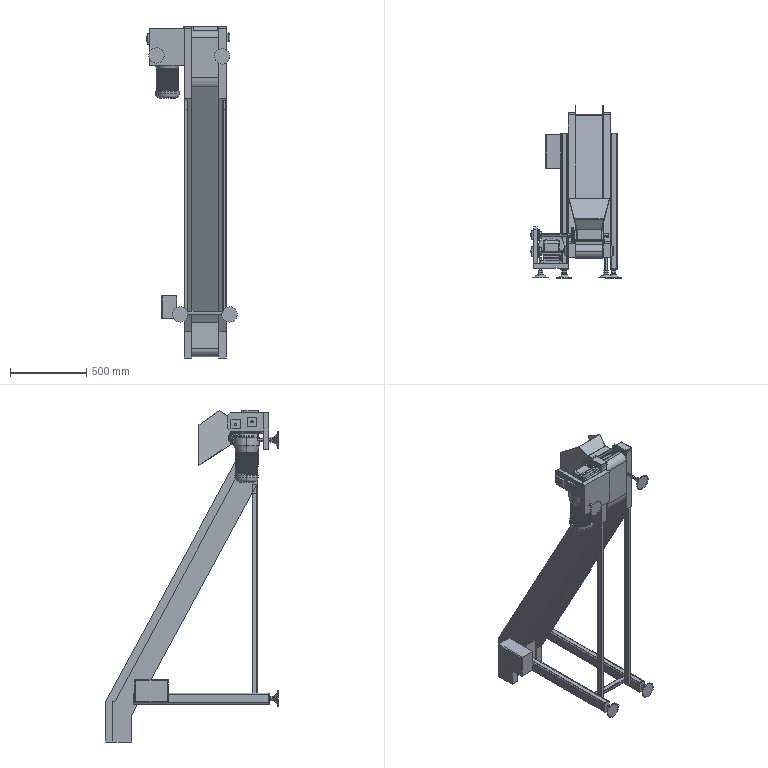Part | NX | 63 solids | 2674 faces | box 593.919 x 1135 x 2179 mm | volume 55419513 mm3 | plane 1476 | cylinder 807 | cone 278 | torus 110 | spline 3 | commonest cylinder face diameters 43.92 x152 3.6 x86 5.709 x86 81.984 x74 95.16 x72 7.62 x52